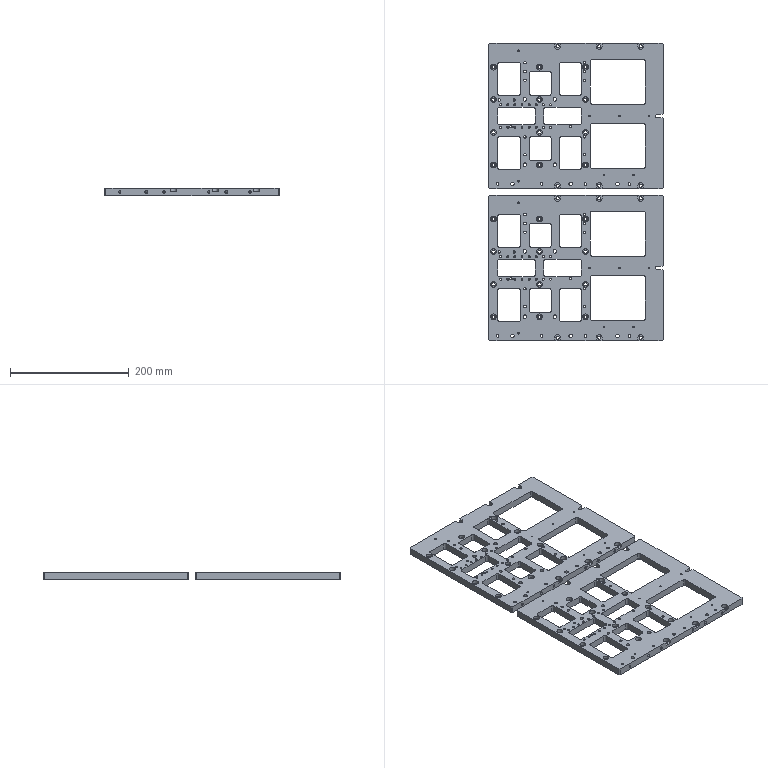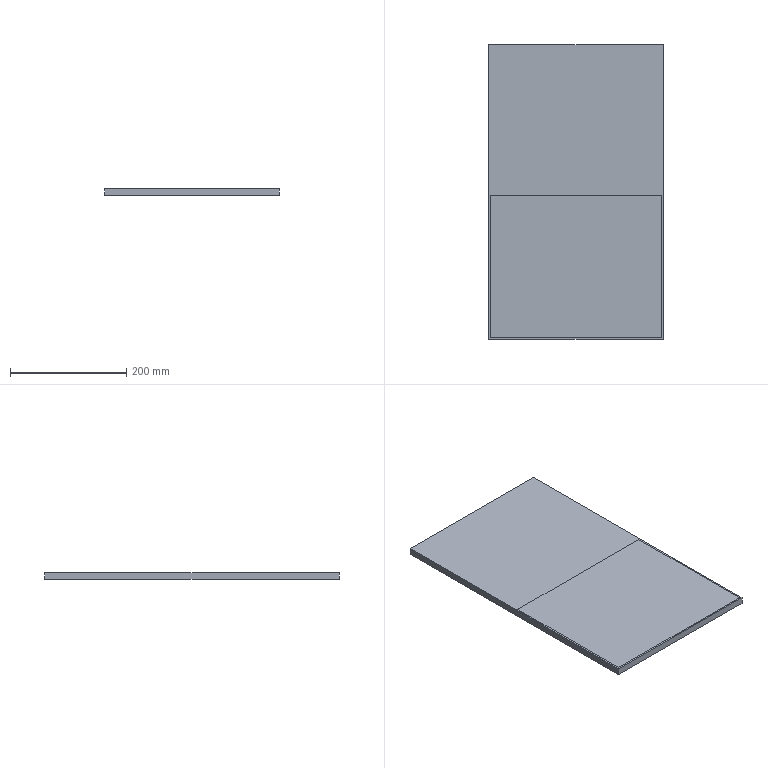CAM job | NX | 3+2 milling, drilling | part box 294 x 501 x 12 mm | stock box 300 x 507 x 12 mm
Tools:
number,name,description,diameter,corner_radius,flute_length,length,flutes
22,D6A45,Milling Tool-5 Parameters,6.0,0.0,3.0,3.0,2
3,3.3ZT,Drilling Tool,3.2,0.0,35.0,50.0,2
20,D10,Milling Tool-5 Parameters,10.0,0.0,50.0,75.0,2
15,D4,Milling Tool-5 Parameters,4.0,0.0,50.0,75.0,2
13,D3,Milling Tool-5 Parameters,3.0,0.0,50.0,75.0,2
11,D10JING,Milling Tool-5 Parameters,10.0,0.0,50.0,75.0,2
21,4.1ZT,Drilling Tool,4.2,0.0,35.0,50.0,2
1,5.5ZT,Drilling Tool,5.5,0.0,35.0,50.0,2
2,2.5ZT,Drilling Tool,2.5,0.0,35.0,50.0,2
17,D6,Milling Tool-5 Parameters,6.0,0.0,50.0,75.0,2
Operations:
program,operation,operation_type,tool,method,geometry_group,spindle_rpm,surface_speed,feed_per_tooth,feed_cut,feed_plunge,cut_length_mm,path_length_mm,cut_time_min,machine_time_min
1AB胶-505-300-12毛胚,DRILLING_COPY_1_COPY_1,Operation,D6A45,METHOD,A,5000.0,94.0,0.025,250.0,0.0,528.0,4774.03,2.112,2.537
1AB胶-505-300-12毛胚,DRILLING_COPY_1_COPY_COPY_COPY_COPY_1_COPY_COPY_1_COPY_COPY_1,Operation,4.1ZT,METHOD,A,2000.0,20.0,0.0375,150.0,0.0,414.283,2349.375,2.762,2.955
1AB胶-505-300-12毛胚,DRILLING_COPY_1_COPY_COPY_COPY_COPY_1_COPY_COPY_1_COPY_COPY_1_COPY_1,Operation,5.5ZT,METHOD,A,2000.0,20.0,0.0375,150.0,0.0,635.485,3472.668,4.237,4.52
1AB胶-505-300-12毛胚,DRILLING_COPY_1_COPY_COPY_COPY_COPY_1_COPY_COPY_1_COPY_COPY_1_COPY_1_COPY,Operation,5.5ZT,METHOD,A,2000.0,20.0,0.0375,150.0,0.0,247.133,1549.482,1.648,1.778
1AB胶-505-300-12毛胚,DRILLING_COPY_1_COPY_COPY_COPY_COPY_1_COPY_COPY_1_COPY_COPY_1_COPY,Operation,3.3ZT,METHOD,A,2000.0,20.0,0.0375,150.0,0.0,542.764,1879.126,3.618,3.752
1AB胶-505-300-12毛胚,DRILLING_COPY_1_COPY_COPY_COPY_COPY_1_COPY_COPY_1_COPY_COPY_1_COPY_COPY,Operation,3.3ZT,METHOD,A,2000.0,20.0,0.0375,150.0,0.0,203.536,1308.148,1.357,1.467
1AB胶-505-300-12毛胚,DRILLING_COPY_1_COPY_COPY_COPY_COPY_1_COPY_COPY_1_COPY_COPY_1_COPY_COPY_COPY,Operation,2.5ZT,METHOD,A,2000.0,20.0,0.0375,150.0,0.0,234.515,1724.922,1.563,1.712
1AB胶-505-300-12毛胚,ZLEVEL_PROFILE_COPY,ZLevelMilling,D10,METHOD,A,7500.0,235.0,0.1667,2500.0,100.0,33395.966,34068.42,13.358,13.426
1AB胶-505-300-12毛胚,ZLEVEL_PROFILE_COPY_COPY_2,ZLevelMilling,D10,METHOD,A,7500.0,235.0,0.1667,2500.0,100.0,52311.59,55858.836,20.925,21.279
1AB胶-505-300-12毛胚,ZLEVEL_PROFILE_COPY_COPY_2_1_COPY_3,ZLevelMilling,D6,METHOD,A,7501.0,94.0,0.0933,1400.0,100.0,4592.844,6921.05,3.281,3.513
1AB胶-505-300-12毛胚,HOLE_MILLING_COPY,CylinderMilling,D6,METHOD,A,7500.0,141.0,0.0933,1400.0,100.0,4978.574,7929.574,3.556,3.851
1AB胶-505-300-12毛胚,ZLEVEL_PROFILE_COPY_COPY_2_1,ZLevelMilling,D4,METHOD,A,7501.0,94.0,0.0933,1400.0,100.0,17844.545,36813.865,12.746,14.643
1AB胶-505-300-12毛胚,ZLEVEL_PROFILE_COPY_COPY_2_1_COPY_2,ZLevelMilling,D4,METHOD,A,7501.0,94.0,0.0933,1400.0,100.0,1571.749,2201.809,1.123,1.186
1AB胶-505-300-12毛胚,ZLEVEL_PROFILE_COPY_COPY_2_1_COPY_1,ZLevelMilling,D4,METHOD,A,7501.0,94.0,0.0667,1000.0,100.0,7746.146,11977.572,7.746,8.169
1AB胶-505-300-12毛胚,HOLE_MILLING_COPY_COPY_COPY,CylinderMilling,D4,METHOD,A,7500.0,70.0,0.0667,1000.0,100.0,2598.938,4639.491,2.599,2.803
1AB胶-505-300-12毛胚,HOLE_MILLING_COPY_COPY,CylinderMilling,D3,METHOD,A,7500.0,70.0,0.0667,1000.0,100.0,1936.153,3640.744,1.936,2.107
1AB胶-505-300-12毛胚,ZLEVEL_PROFILE_1_COPY_1_COPY_COPY,ZLevelMilling,D6A45,METHOD,A,7500.0,141.0,0.0667,1000.0,100.0,8175.551,29371.541,8.176,10.295
1AB胶-505-300-12毛胚,刀补15,CylinderMilling,D4,METHOD,A,7500.0,70.0,0.0667,1000.0,100.0,676.465,2717.018,0.6765,0.8805
1AB胶-505-300-12毛胚,刀补12_1,ZLevelMilling,D4,METHOD,A,7500.0,47.0,0.0667,1000.0,100.0,190.286,622.038,0.1903,0.2335
1AB胶-505-300-12毛胚,刀补13,CylinderMilling,D3,METHOD,A,7500.0,70.0,0.0667,1000.0,100.0,370.782,2075.372,0.3708,0.5412
1AB胶-505-300-12毛胚,ZLEVEL_PROFILE_COPY_COPY_1,ZLevelMilling,D10JING,METHOD,A,7500.0,235.0,0.0667,1000.0,100.0,6721.054,7444.962,6.721,6.793
2,DRILLING_COPY_1_COPY_1_COPY,Operation,D6A45,METHOD,B,5000.0,94.0,0.025,250.0,0.0,24.0,658.242,0.096,0.1594
2,DRILLING_COPY_1_COPY_COPY_COPY_COPY_1_COPY_COPY_1_COPY_COPY_1_COPY_2,Operation,4.1ZT,METHOD,B,2000.0,20.0,0.0375,150.0,0.0,94.052,658.433,0.627,0.6834
2,HOLE_MILLING_COPY_COPY_COPY_COPY,CylinderMilling,D3,METHOD,B,7500.0,70.0,0.0667,1000.0,100.0,413.362,687.362,0.4134,0.4408
2,ZLEVEL_PROFILE_1_COPY_1_COPY_COPY_COPY,ZLevelMilling,D6A45,METHOD,B,7500.0,141.0,0.0667,1000.0,100.0,73.101,840.553,0.0731,0.1498
2,刀补15_COPY,CylinderMilling,D3,METHOD,B,7500.0,70.0,0.0667,1000.0,100.0,84.047,358.048,0.084,0.1114